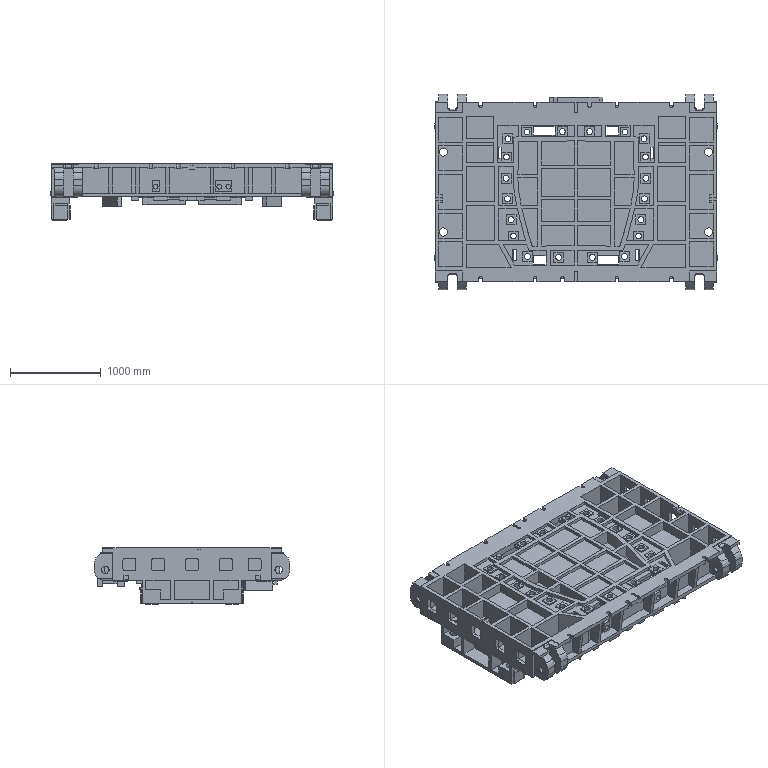Part | NX | features solid 2 | 1 solid | 1687 faces | box 3110 x 2150 x 625 mm | volume 777737805 mm3 | plane 1390 | cylinder 251 | spline 38 | torus 8 | commonest cylinder face diameters 40 x86 83 x48 65 x20 79 x16 30 x14 80 x10